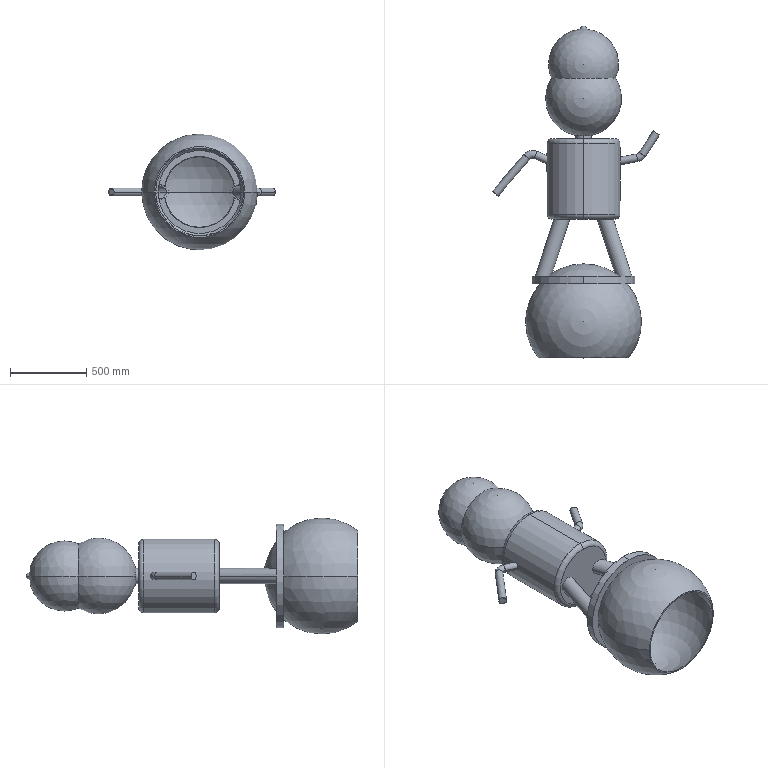Part | SolidWorks | features Sweep 4, ICE 3, Revolution 2, CombineBodies 1, Fillet 1, Shell 1 | 1 solid | 85 faces | box 1093 x 2171 x 758 mm | volume 26788411 mm3 | cylinder 36 | sphere 20 | torus 16 | plane 13 | commonest cylinder face diameters 37.08 x8 50 x8 87.08 x6 100 x6 466.08 x2 479 x2